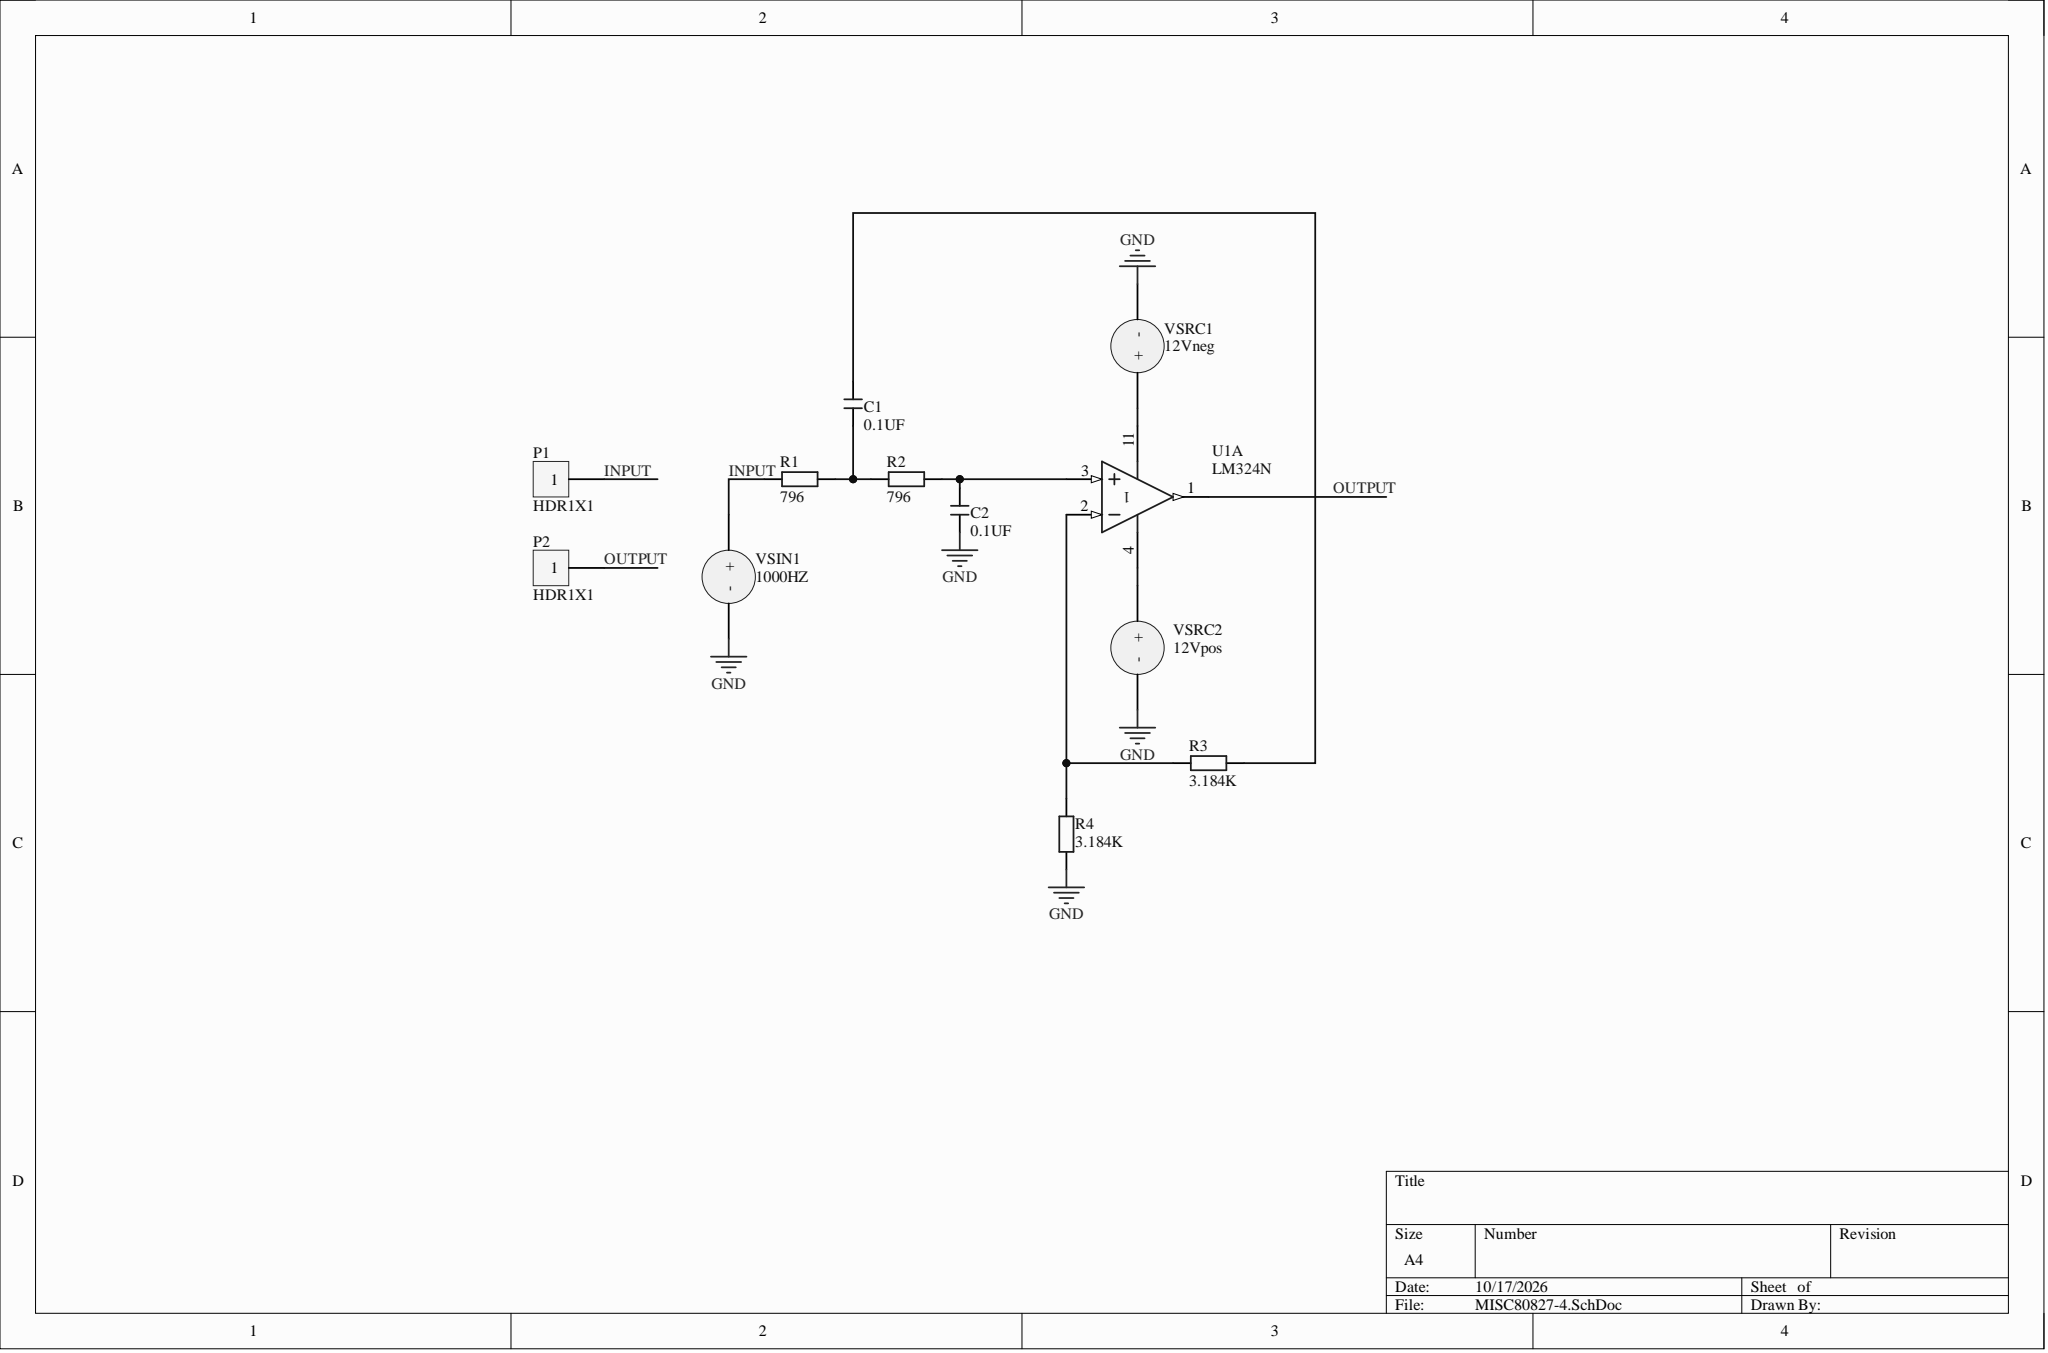Circuit board | Altium Designer | 12 parts | 9 nets
Bill of materials:
Comment,Description,Designator,Footprint,LibRef,Quantity
"0.1UF","Monolithic ceramic capacitor","C1, C2","MLCC5.08-A","C-MLCC","2"
"HDR1X1","","P1, P2","HDR1X1","HDR1X1","2"
"796","Color-band resistor","R1, R2","RS 1/4W","R-S","2"
"3.184K","Color-band resistor","R3, R4","RS 1/4W","R-S","2"
"LM324N","Quad Low-Power Operational Amplifier","U1","646-06","LM324N","1"
"1000HZ","","VSIN1","HDR1X2","电流源","1"
"12Vneg","","VSRC1","HDR1X2","电流源","1"
"12Vpos","","VSRC2","HDR1X2","电流源","1"
Netlist (Protel format):
[
C1
MLCC5.08-A
0.1UF



]
[
C2
MLCC5.08-A
0.1UF



]
[
P1
HDR1X1
HDR1X1



]
[
P2
HDR1X1
HDR1X1



]
[
R1
RS 1/4W
796



]
[
R2
RS 1/4W
796



]
[
R3
RS 1/4W
3.184K



]
[
R4
RS 1/4W
3.184K



]
[
U1
646-06
LM324N



]
[
VSIN1
HDR1X2
1000HZ



]
[
VSRC1
HDR1X2
12Vneg



]
[
VSRC2
HDR1X2
12Vpos



]
(
OUTPUT
P2-1
U1-1
)
(
NetU1_11
U1-11
VSRC1-1
)
(
NetU1_4
U1-4
VSRC2-1
)
(
NetR3_2
R3-2
R4-2
U1-2
)
(
NetC2_2
C2-2
R2-2
U1-3
)
(
NetC1_2
C1-2
R3-1
)
(
NetC1_1
C1-1
R1-2
R2-1
)
(
INPUT
P1-1
R1-1
VSIN1-1
)
(
GND
C2-1
R4-1
VSIN1-2
VSRC1-2
VSRC2-2
)